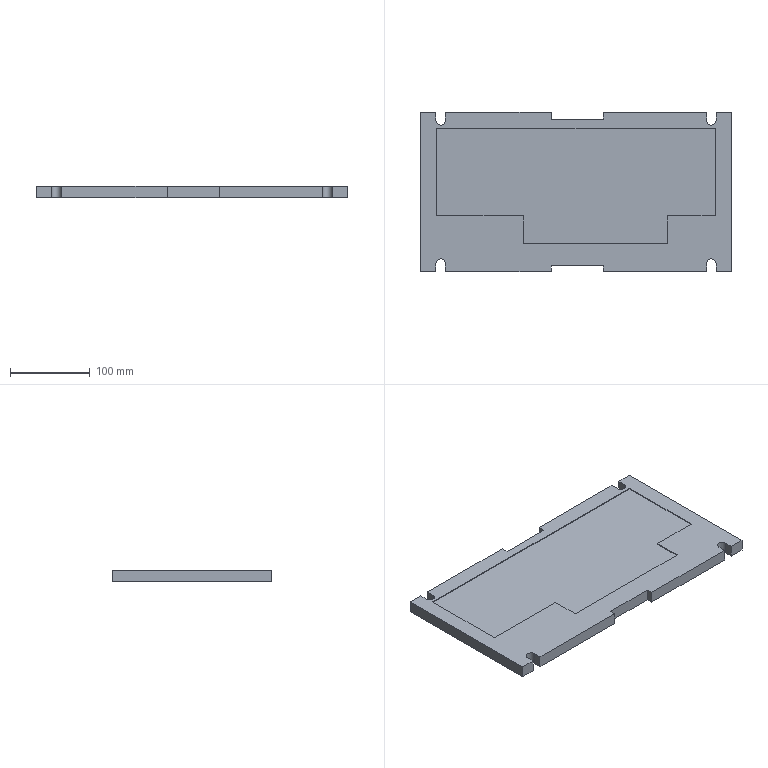Part | STEP file | MYT-A01-P07 | 1 solid | 39 faces | box 390 x 200 x 15 mm | volume 1098768 mm3 | plane 35 | cylinder 4 | commonest cylinder face diameters 12 x4
STEP:
#1=CARTESIAN_POINT('',(-31.137,100.,0.));
#2=VERTEX_POINT('',#1);
#3=CARTESIAN_POINT('',(-164.,100.,0.));
#4=VERTEX_POINT('',#3);
#5=CARTESIAN_POINT('',(-195.,100.,0.));
#6=DIRECTION('',(-1.,0.,0.));
#7=VECTOR('',#6,1000.);
#8=LINE('',#5,#7);
#9=EDGE_CURVE('',#2,#4,#8,.T.);
#10=ORIENTED_EDGE('',*,*,#9,.T.);
#11=CARTESIAN_POINT('',(-164.,100.,15.));
#12=VERTEX_POINT('',#11);
#13=CARTESIAN_POINT('',(-164.,100.,15.));
#14=DIRECTION('',(0.,0.,1.));
#15=VECTOR('',#14,1000.);
#16=LINE('',#13,#15);
#17=EDGE_CURVE('',#4,#12,#16,.T.);
#18=ORIENTED_EDGE('',*,*,#17,.T.);
#19=CARTESIAN_POINT('',(-31.137,100.,15.));
#20=VERTEX_POINT('',#19);
#21=CARTESIAN_POINT('',(-195.,100.,15.));
#22=DIRECTION('',(-1.,0.,0.));
#23=VECTOR('',#22,1000.);
#24=LINE('',#21,#23);
#25=EDGE_CURVE('',#20,#12,#24,.T.);
#26=ORIENTED_EDGE('',*,*,#25,.F.);
#27=CARTESIAN_POINT('',(-31.137,100.,15.));
#28=DIRECTION('',(0.,0.,-1.));
#29=VECTOR('',#28,1000.);
#30=LINE('',#27,#29);
#31=EDGE_CURVE('',#20,#2,#30,.T.);
#32=ORIENTED_EDGE('',*,*,#31,.T.);
#33=EDGE_LOOP('',(#10,#18,#26,#32));
#34=FACE_OUTER_BOUND('',#33,.T.);
#35=CARTESIAN_POINT('',(-195.,100.,15.));
#36=DIRECTION('',(0.,-1.,0.));
#37=DIRECTION('',(0.,0.,-1.));
#38=AXIS2_PLACEMENT_3D('',#35,#36,#37);
#39=PLANE('',#38);
#40=ADVANCED_FACE('',(#34),#39,.F.);
#41=CARTESIAN_POINT('',(-195.,-100.,0.));
#42=VERTEX_POINT('',#41);
#43=CARTESIAN_POINT('',(-176.,-100.,0.));
#44=VERTEX_POINT('',#43);
#45=CARTESIAN_POINT('',(-195.,-100.,0.));
#46=DIRECTION('',(1.,0.,0.));
#47=VECTOR('',#46,1000.);
#48=LINE('',#45,#47);
#49=EDGE_CURVE('',#42,#44,#48,.T.);
#50=ORIENTED_EDGE('',*,*,#49,.T.);
#51=CARTESIAN_POINT('',(-176.,-100.,15.));
#52=VERTEX_POINT('',#51);
#53=CARTESIAN_POINT('',(-176.,-100.,15.));
#54=DIRECTION('',(0.,0.,1.));
#55=VECTOR('',#54,1000.);
#56=LINE('',#53,#55);
#57=EDGE_CURVE('',#44,#52,#56,.T.);
#58=ORIENTED_EDGE('',*,*,#57,.T.);
#59=CARTESIAN_POINT('',(-195.,-100.,15.));
#60=VERTEX_POINT('',#59);
#61=CARTESIAN_POINT('',(-195.,-100.,15.));
#62=DIRECTION('',(1.,0.,0.));
#63=VECTOR('',#62,1000.);
#64=LINE('',#61,#63);
#65=EDGE_CURVE('',#60,#52,#64,.T.);
#66=ORIENTED_EDGE('',*,*,#65,.F.);
#67=CARTESIAN_POINT('',(-195.,-100.,15.));
#68=DIRECTION('',(0.,0.,-1.));
#69=VECTOR('',#68,1000.);
#70=LINE('',#67,#69);
#71=EDGE_CURVE('',#60,#42,#70,.T.);
#72=ORIENTED_EDGE('',*,*,#71,.T.);
#73=EDGE_LOOP('',(#50,#58,#66,#72));
#74=FACE_OUTER_BOUND('',#73,.T.);
#75=CARTESIAN_POINT('',(-195.,-100.,15.));
#76=DIRECTION('',(0.,1.,0.));
#77=DIRECTION('',(0.,0.,1.));
#78=AXIS2_PLACEMENT_3D('',#75,#76,#77);
#79=PLANE('',#78);
#80=ADVANCED_FACE('',(#74),#79,.F.);
#81=CARTESIAN_POINT('',(195.,100.,0.));
#82=VERTEX_POINT('',#81);
#83=CARTESIAN_POINT('',(176.,100.,0.));
#84=VERTEX_POINT('',#83);
#85=CARTESIAN_POINT('',(-195.,100.,0.));
#86=DIRECTION('',(-1.,0.,0.));
#87=VECTOR('',#86,1000.);
#88=LINE('',#85,#87);
#89=EDGE_CURVE('',#82,#84,#88,.T.);
#90=ORIENTED_EDGE('',*,*,#89,.T.);
#91=CARTESIAN_POINT('',(176.,100.,15.));
#92=VERTEX_POINT('',#91);
#93=CARTESIAN_POINT('',(176.,100.,15.));
#94=DIRECTION('',(0.,0.,1.));
#95=VECTOR('',#94,1000.);
#96=LINE('',#93,#95);
#97=EDGE_CURVE('',#84,#92,#96,.T.);
#98=ORIENTED_EDGE('',*,*,#97,.T.);
#99=CARTESIAN_POINT('',(195.,100.,15.));
#100=VERTEX_POINT('',#99);
#101=CARTESIAN_POINT('',(-195.,100.,15.));
#102=DIRECTION('',(-1.,0.,0.));
#103=VECTOR('',#102,1000.);
#104=LINE('',#101,#103);
#105=EDGE_CURVE('',#100,#92,#104,.T.);
#106=ORIENTED_EDGE('',*,*,#105,.F.);
#107=CARTESIAN_POINT('',(195.,100.,15.));
#108=DIRECTION('',(0.,0.,-1.));
#109=VECTOR('',#108,1000.);
#110=LINE('',#107,#109);
#111=EDGE_CURVE('',#100,#82,#110,.T.);
#112=ORIENTED_EDGE('',*,*,#111,.T.);
#113=EDGE_LOOP('',(#90,#98,#106,#112));
#114=FACE_OUTER_BOUND('',#113,.T.);
#115=CARTESIAN_POINT('',(-195.,100.,15.));
#116=DIRECTION('',(0.,-1.,0.));
#117=DIRECTION('',(0.,0.,-1.));
#118=AXIS2_PLACEMENT_3D('',#115,#116,#117);
#119=PLANE('',#118);
#120=ADVANCED_FACE('',(#114),#119,.F.);
#121=CARTESIAN_POINT('',(34.454,-100.,0.));
#122=VERTEX_POINT('',#121);
#123=CARTESIAN_POINT('',(164.,-100.,0.));
#124=VERTEX_POINT('',#123);
#125=CARTESIAN_POINT('',(-195.,-100.,0.));
#126=DIRECTION('',(1.,0.,0.));
#127=VECTOR('',#126,1000.);
#128=LINE('',#125,#127);
#129=EDGE_CURVE('',#122,#124,#128,.T.);
#130=ORIENTED_EDGE('',*,*,#129,.T.);
#131=CARTESIAN_POINT('',(164.,-100.,15.));
#132=VERTEX_POINT('',#131);
#133=CARTESIAN_POINT('',(164.,-100.,15.));
#134=DIRECTION('',(0.,0.,1.));
#135=VECTOR('',#134,1000.);
#136=LINE('',#133,#135);
#137=EDGE_CURVE('',#124,#132,#136,.T.);
#138=ORIENTED_EDGE('',*,*,#137,.T.);
#139=CARTESIAN_POINT('',(34.454,-100.,15.));
#140=VERTEX_POINT('',#139);
#141=CARTESIAN_POINT('',(-195.,-100.,15.));
#142=DIRECTION('',(1.,0.,0.));
#143=VECTOR('',#142,1000.);
#144=LINE('',#141,#143);
#145=EDGE_CURVE('',#140,#132,#144,.T.);
#146=ORIENTED_EDGE('',*,*,#145,.F.);
#147=CARTESIAN_POINT('',(34.454,-100.,15.));
#148=DIRECTION('',(0.,0.,-1.));
#149=VECTOR('',#148,1000.);
#150=LINE('',#147,#149);
#151=EDGE_CURVE('',#140,#122,#150,.T.);
#152=ORIENTED_EDGE('',*,*,#151,.T.);
#153=EDGE_LOOP('',(#130,#138,#146,#152));
#154=FACE_OUTER_BOUND('',#153,.T.);
#155=CARTESIAN_POINT('',(-195.,-100.,15.));
#156=DIRECTION('',(0.,1.,0.));
#157=DIRECTION('',(0.,0.,1.));
#158=AXIS2_PLACEMENT_3D('',#155,#156,#157);
#159=PLANE('',#158);
#160=ADVANCED_FACE('',(#154),#159,.F.);
#161=CARTESIAN_POINT('',(-176.,100.,15.));
#162=VERTEX_POINT('',#161);
#163=CARTESIAN_POINT('',(-195.,100.,15.));
#164=VERTEX_POINT('',#163);
#165=CARTESIAN_POINT('',(-195.,100.,15.));
#166=DIRECTION('',(-1.,0.,0.));
#167=VECTOR('',#166,1000.);
#168=LINE('',#165,#167);
#169=EDGE_CURVE('',#162,#164,#168,.T.);
#170=ORIENTED_EDGE('',*,*,#169,.F.);
#171=CARTESIAN_POINT('',(-176.,100.,0.));
#172=VERTEX_POINT('',#171);
#173=CARTESIAN_POINT('',(-176.,100.,15.));
#174=DIRECTION('',(0.,0.,-1.));
#175=VECTOR('',#174,1000.);
#176=LINE('',#173,#175);
#177=EDGE_CURVE('',#162,#172,#176,.T.);
#178=ORIENTED_EDGE('',*,*,#177,.T.);
#179=CARTESIAN_POINT('',(-195.,100.,0.));
#180=VERTEX_POINT('',#179);
#181=CARTESIAN_POINT('',(-195.,100.,0.));
#182=DIRECTION('',(-1.,0.,0.));
#183=VECTOR('',#182,1000.);
#184=LINE('',#181,#183);
#185=EDGE_CURVE('',#172,#180,#184,.T.);
#186=ORIENTED_EDGE('',*,*,#185,.T.);
#187=CARTESIAN_POINT('',(-195.,100.,15.));
#188=DIRECTION('',(0.,0.,-1.));
#189=VECTOR('',#188,1000.);
#190=LINE('',#187,#189);
#191=EDGE_CURVE('',#164,#180,#190,.T.);
#192=ORIENTED_EDGE('',*,*,#191,.F.);
#193=EDGE_LOOP('',(#170,#178,#186,#192));
#194=FACE_OUTER_BOUND('',#193,.T.);
#195=CARTESIAN_POINT('',(-195.,100.,15.));
#196=DIRECTION('',(0.,-1.,0.));
#197=DIRECTION('',(0.,0.,-1.));
#198=AXIS2_PLACEMENT_3D('',#195,#196,#197);
#199=PLANE('',#198);
#200=ADVANCED_FACE('',(#194),#199,.F.);
#201=CARTESIAN_POINT('',(-164.,-100.,15.));
#202=VERTEX_POINT('',#201);
#203=CARTESIAN_POINT('',(-31.137,-100.,15.));
#204=VERTEX_POINT('',#203);
#205=CARTESIAN_POINT('',(-195.,-100.,15.));
#206=DIRECTION('',(1.,0.,0.));
#207=VECTOR('',#206,1000.);
#208=LINE('',#205,#207);
#209=EDGE_CURVE('',#202,#204,#208,.T.);
#210=ORIENTED_EDGE('',*,*,#209,.F.);
#211=CARTESIAN_POINT('',(-164.,-100.,0.));
#212=VERTEX_POINT('',#211);
#213=CARTESIAN_POINT('',(-164.,-100.,15.));
#214=DIRECTION('',(0.,0.,-1.));
#215=VECTOR('',#214,1000.);
#216=LINE('',#213,#215);
#217=EDGE_CURVE('',#202,#212,#216,.T.);
#218=ORIENTED_EDGE('',*,*,#217,.T.);
#219=CARTESIAN_POINT('',(-31.137,-100.,0.));
#220=VERTEX_POINT('',#219);
#221=CARTESIAN_POINT('',(-195.,-100.,0.));
#222=DIRECTION('',(1.,0.,0.));
#223=VECTOR('',#222,1000.);
#224=LINE('',#221,#223);
#225=EDGE_CURVE('',#212,#220,#224,.T.);
#226=ORIENTED_EDGE('',*,*,#225,.T.);
#227=CARTESIAN_POINT('',(-31.137,-100.,15.));
#228=DIRECTION('',(0.,0.,1.));
#229=VECTOR('',#228,1000.);
#230=LINE('',#227,#229);
#231=EDGE_CURVE('',#220,#204,#230,.T.);
#232=ORIENTED_EDGE('',*,*,#231,.T.);
#233=EDGE_LOOP('',(#210,#218,#226,#232));
#234=FACE_OUTER_BOUND('',#233,.T.);
#235=CARTESIAN_POINT('',(-195.,-100.,15.));
#236=DIRECTION('',(0.,1.,0.));
#237=DIRECTION('',(0.,0.,1.));
#238=AXIS2_PLACEMENT_3D('',#235,#236,#237);
#239=PLANE('',#238);
#240=ADVANCED_FACE('',(#234),#239,.F.);
#241=CARTESIAN_POINT('',(195.,-100.,0.));
#242=VERTEX_POINT('',#241);
#243=CARTESIAN_POINT('',(195.,100.,0.));
#244=DIRECTION('',(0.,1.,0.));
#245=VECTOR('',#244,1000.);
#246=LINE('',#243,#245);
#247=EDGE_CURVE('',#242,#82,#246,.T.);
#248=ORIENTED_EDGE('',*,*,#247,.T.);
#249=ORIENTED_EDGE('',*,*,#111,.F.);
#250=CARTESIAN_POINT('',(195.,-100.,15.));
#251=VERTEX_POINT('',#250);
#252=CARTESIAN_POINT('',(195.,100.,15.));
#253=DIRECTION('',(0.,1.,0.));
#254=VECTOR('',#253,1000.);
#255=LINE('',#252,#254);
#256=EDGE_CURVE('',#251,#100,#255,.T.);
#257=ORIENTED_EDGE('',*,*,#256,.F.);
#258=CARTESIAN_POINT('',(195.,-100.,15.));
#259=DIRECTION('',(0.,0.,-1.));
#260=VECTOR('',#259,1000.);
#261=LINE('',#258,#260);
#262=EDGE_CURVE('',#251,#242,#261,.T.);
#263=ORIENTED_EDGE('',*,*,#262,.T.);
#264=EDGE_LOOP('',(#248,#249,#257,#263));
#265=FACE_OUTER_BOUND('',#264,.T.);
#266=CARTESIAN_POINT('',(195.,100.,15.));
#267=DIRECTION('',(-1.,0.,0.));
#268=DIRECTION('',(0.,0.,1.));
#269=AXIS2_PLACEMENT_3D('',#266,#267,#268);
#270=PLANE('',#269);
#271=ADVANCED_FACE('',(#265),#270,.F.);
#272=CARTESIAN_POINT('',(164.,100.,15.));
#273=VERTEX_POINT('',#272);
#274=CARTESIAN_POINT('',(34.454,100.,15.));
#275=VERTEX_POINT('',#274);
#276=CARTESIAN_POINT('',(-195.,100.,15.));
#277=DIRECTION('',(-1.,0.,0.));
#278=VECTOR('',#277,1000.);
#279=LINE('',#276,#278);
#280=EDGE_CURVE('',#273,#275,#279,.T.);
#281=ORIENTED_EDGE('',*,*,#280,.F.);
#282=CARTESIAN_POINT('',(164.,100.,0.));
#283=VERTEX_POINT('',#282);
#284=CARTESIAN_POINT('',(164.,100.,15.));
#285=DIRECTION('',(0.,0.,-1.));
#286=VECTOR('',#285,1000.);
#287=LINE('',#284,#286);
#288=EDGE_CURVE('',#273,#283,#287,.T.);
#289=ORIENTED_EDGE('',*,*,#288,.T.);
#290=CARTESIAN_POINT('',(34.454,100.,0.));
#291=VERTEX_POINT('',#290);
#292=CARTESIAN_POINT('',(-195.,100.,0.));
#293=DIRECTION('',(-1.,0.,0.));
#294=VECTOR('',#293,1000.);
#295=LINE('',#292,#294);
#296=EDGE_CURVE('',#283,#291,#295,.T.);
#297=ORIENTED_EDGE('',*,*,#296,.T.);
#298=CARTESIAN_POINT('',(34.454,100.,15.));
#299=DIRECTION('',(0.,0.,1.));
#300=VECTOR('',#299,1000.);
#301=LINE('',#298,#300);
#302=EDGE_CURVE('',#291,#275,#301,.T.);
#303=ORIENTED_EDGE('',*,*,#302,.T.);
#304=EDGE_LOOP('',(#281,#289,#297,#303));
#305=FACE_OUTER_BOUND('',#304,.T.);
#306=CARTESIAN_POINT('',(-195.,100.,15.));
#307=DIRECTION('',(0.,-1.,0.));
#308=DIRECTION('',(0.,0.,-1.));
#309=AXIS2_PLACEMENT_3D('',#306,#307,#308);
#310=PLANE('',#309);
#311=ADVANCED_FACE('',(#305),#310,.F.);
#312=CARTESIAN_POINT('',(-195.,100.,0.));
#313=DIRECTION('',(0.,-1.,0.));
#314=VECTOR('',#313,1000.);
#315=LINE('',#312,#314);
#316=EDGE_CURVE('',#180,#42,#315,.T.);
#317=ORIENTED_EDGE('',*,*,#316,.T.);
#318=ORIENTED_EDGE('',*,*,#71,.F.);
#319=CARTESIAN_POINT('',(-195.,100.,15.));
#320=DIRECTION('',(0.,-1.,0.));
#321=VECTOR('',#320,1000.);
#322=LINE('',#319,#321);
#323=EDGE_CURVE('',#164,#60,#322,.T.);
#324=ORIENTED_EDGE('',*,*,#323,.F.);
#325=ORIENTED_EDGE('',*,*,#191,.T.);
#326=EDGE_LOOP('',(#317,#318,#324,#325));
#327=FACE_OUTER_BOUND('',#326,.T.);
#328=CARTESIAN_POINT('',(-195.,100.,15.));
#329=DIRECTION('',(1.,0.,0.));
#330=DIRECTION('',(0.,1.,0.));
#331=AXIS2_PLACEMENT_3D('',#328,#329,#330);
#332=PLANE('',#331);
#333=ADVANCED_FACE('',(#327),#332,.F.);
#334=CARTESIAN_POINT('',(176.,-100.,15.));
#335=VERTEX_POINT('',#334);
#336=CARTESIAN_POINT('',(-195.,-100.,15.));
#337=DIRECTION('',(1.,0.,0.));
#338=VECTOR('',#337,1000.);
#339=LINE('',#336,#338);
#340=EDGE_CURVE('',#335,#251,#339,.T.);
#341=ORIENTED_EDGE('',*,*,#340,.F.);
#342=CARTESIAN_POINT('',(176.,-100.,0.));
#343=VERTEX_POINT('',#342);
#344=CARTESIAN_POINT('',(176.,-100.,15.));
#345=DIRECTION('',(0.,0.,-1.));
#346=VECTOR('',#345,1000.);
#347=LINE('',#344,#346);
#348=EDGE_CURVE('',#335,#343,#347,.T.);
#349=ORIENTED_EDGE('',*,*,#348,.T.);
#350=CARTESIAN_POINT('',(-195.,-100.,0.));
#351=DIRECTION('',(1.,0.,0.));
#352=VECTOR('',#351,1000.);
#353=LINE('',#350,#352);
#354=EDGE_CURVE('',#343,#242,#353,.T.);
#355=ORIENTED_EDGE('',*,*,#354,.T.);
#356=ORIENTED_EDGE('',*,*,#262,.F.);
#357=EDGE_LOOP('',(#341,#349,#355,#356));
#358=FACE_OUTER_BOUND('',#357,.T.);
#359=CARTESIAN_POINT('',(-195.,-100.,15.));
#360=DIRECTION('',(0.,1.,0.));
#361=DIRECTION('',(0.,0.,1.));
#362=AXIS2_PLACEMENT_3D('',#359,#360,#361);
#363=PLANE('',#362);
#364=ADVANCED_FACE('',(#358),#363,.F.);
#365=CARTESIAN_POINT('',(-176.,-90.,15.));
#366=VERTEX_POINT('',#365);
#367=CARTESIAN_POINT('',(-176.,-110.,15.));
#368=DIRECTION('',(0.,-1.,0.));
#369=VECTOR('',#368,1000.);
#370=LINE('',#367,#369);
#371=EDGE_CURVE('',#366,#52,#370,.T.);
#372=ORIENTED_EDGE('',*,*,#371,.F.);
#373=CARTESIAN_POINT('',(-164.,-90.,15.));
#374=VERTEX_POINT('',#373);
#375=CARTESIAN_POINT('',(-170.,-90.,15.));
#376=DIRECTION('',(0.,0.,1.));
#377=DIRECTION('',(-1.,0.,0.));
#378=AXIS2_PLACEMENT_3D('',#375,#376,#377);
#379=CIRCLE('',#378,6.);
#380=EDGE_CURVE('',#374,#366,#379,.T.);
#381=ORIENTED_EDGE('',*,*,#380,.F.);
#382=CARTESIAN_POINT('',(-164.,-110.,15.));
#383=DIRECTION('',(0.,1.,0.));
#384=VECTOR('',#383,1000.);
#385=LINE('',#382,#384);
#386=EDGE_CURVE('',#202,#374,#385,.T.);
#387=ORIENTED_EDGE('',*,*,#386,.F.);
#388=ORIENTED_EDGE('',*,*,#209,.T.);
#389=CARTESIAN_POINT('',(-31.137,-92.567,15.));
#390=VERTEX_POINT('',#389);
#391=CARTESIAN_POINT('',(-31.137,-118.233,15.));
#392=DIRECTION('',(0.,-1.,0.));
#393=VECTOR('',#392,1000.);
#394=LINE('',#391,#393);
#395=EDGE_CURVE('',#390,#204,#394,.T.);
#396=ORIENTED_EDGE('',*,*,#395,.F.);
#397=CARTESIAN_POINT('',(34.454,-92.567,15.));
#398=VERTEX_POINT('',#397);
#399=CARTESIAN_POINT('',(-31.137,-92.567,15.));
#400=DIRECTION('',(-1.,0.,0.));
#401=VECTOR('',#400,1000.);
#402=LINE('',#399,#401);
#403=EDGE_CURVE('',#398,#390,#402,.T.);
#404=ORIENTED_EDGE('',*,*,#403,.F.);
#405=CARTESIAN_POINT('',(34.454,-118.233,15.));
#406=DIRECTION('',(0.,1.,0.));
#407=VECTOR('',#406,1000.);
#408=LINE('',#405,#407);
#409=EDGE_CURVE('',#140,#398,#408,.T.);
#410=ORIENTED_EDGE('',*,*,#409,.F.);
#411=ORIENTED_EDGE('',*,*,#145,.T.);
#412=CARTESIAN_POINT('',(164.,-90.,15.));
#413=VERTEX_POINT('',#412);
#414=CARTESIAN_POINT('',(164.,-110.,15.));
#415=DIRECTION('',(0.,-1.,0.));
#416=VECTOR('',#415,1000.);
#417=LINE('',#414,#416);
#418=EDGE_CURVE('',#413,#132,#417,.T.);
#419=ORIENTED_EDGE('',*,*,#418,.F.);
#420=CARTESIAN_POINT('',(176.,-90.,15.));
#421=VERTEX_POINT('',#420);
#422=CARTESIAN_POINT('',(170.,-90.,15.));
#423=DIRECTION('',(0.,0.,1.));
#424=DIRECTION('',(-1.,0.,0.));
#425=AXIS2_PLACEMENT_3D('',#422,#423,#424);
#426=CIRCLE('',#425,6.);
#427=EDGE_CURVE('',#421,#413,#426,.T.);
#428=ORIENTED_EDGE('',*,*,#427,.F.);
#429=CARTESIAN_POINT('',(176.,-110.,15.));
#430=DIRECTION('',(0.,1.,0.));
#431=VECTOR('',#430,1000.);
#432=LINE('',#429,#431);
#433=EDGE_CURVE('',#335,#421,#432,.T.);
#434=ORIENTED_EDGE('',*,*,#433,.F.);
#435=ORIENTED_EDGE('',*,*,#340,.T.);
#436=ORIENTED_EDGE('',*,*,#256,.T.);
#437=ORIENTED_EDGE('',*,*,#105,.T.);
#438=CARTESIAN_POINT('',(176.,90.,15.));
#439=VERTEX_POINT('',#438);
#440=CARTESIAN_POINT('',(176.,110.,15.));
#441=DIRECTION('',(0.,1.,0.));
#442=VECTOR('',#441,1000.);
#443=LINE('',#440,#442);
#444=EDGE_CURVE('',#439,#92,#443,.T.);
#445=ORIENTED_EDGE('',*,*,#444,.F.);
#446=CARTESIAN_POINT('',(164.,90.,15.));
#447=VERTEX_POINT('',#446);
#448=CARTESIAN_POINT('',(170.,90.,15.));
#449=DIRECTION('',(0.,0.,1.));
#450=DIRECTION('',(1.,0.,0.));
#451=AXIS2_PLACEMENT_3D('',#448,#449,#450);
#452=CIRCLE('',#451,6.);
#453=EDGE_CURVE('',#447,#439,#452,.T.);
#454=ORIENTED_EDGE('',*,*,#453,.F.);
#455=CARTESIAN_POINT('',(164.,110.,15.));
#456=DIRECTION('',(0.,-1.,0.));
#457=VECTOR('',#456,1000.);
#458=LINE('',#455,#457);
#459=EDGE_CURVE('',#273,#447,#458,.T.);
#460=ORIENTED_EDGE('',*,*,#459,.F.);
#461=ORIENTED_EDGE('',*,*,#280,.T.);
#462=CARTESIAN_POINT('',(34.454,91.372,15.));
#463=VERTEX_POINT('',#462);
#464=CARTESIAN_POINT('',(34.454,110.859,15.));
#465=DIRECTION('',(0.,1.,0.));
#466=VECTOR('',#465,1000.);
#467=LINE('',#464,#466);
#468=EDGE_CURVE('',#463,#275,#467,.T.);
#469=ORIENTED_EDGE('',*,*,#468,.F.);
#470=CARTESIAN_POINT('',(-31.137,91.372,15.));
#471=VERTEX_POINT('',#470);
#472=CARTESIAN_POINT('',(-31.137,91.372,15.));
#473=DIRECTION('',(1.,0.,0.));
#474=VECTOR('',#473,1000.);
#475=LINE('',#472,#474);
#476=EDGE_CURVE('',#471,#463,#475,.T.);
#477=ORIENTED_EDGE('',*,*,#476,.F.);
#478=CARTESIAN_POINT('',(-31.137,110.859,15.));
#479=DIRECTION('',(0.,-1.,0.));
#480=VECTOR('',#479,1000.);
#481=LINE('',#478,#480);
#482=EDGE_CURVE('',#20,#471,#481,.T.);
#483=ORIENTED_EDGE('',*,*,#482,.F.);
#484=ORIENTED_EDGE('',*,*,#25,.T.);
#485=CARTESIAN_POINT('',(-164.,90.,15.));
#486=VERTEX_POINT('',#485);
#487=CARTESIAN_POINT('',(-164.,110.,15.));
#488=DIRECTION('',(0.,1.,0.));
#489=VECTOR('',#488,1000.);
#490=LINE('',#487,#489);
#491=EDGE_CURVE('',#486,#12,#490,.T.);
#492=ORIENTED_EDGE('',*,*,#491,.F.);
#493=CARTESIAN_POINT('',(-176.,90.,15.));
#494=VERTEX_POINT('',#493);
#495=CARTESIAN_POINT('',(-170.,90.,15.));
#496=DIRECTION('',(0.,0.,1.));
#497=DIRECTION('',(1.,0.,0.));
#498=AXIS2_PLACEMENT_3D('',#495,#496,#497);
#499=CIRCLE('',#498,6.);
#500=EDGE_CURVE('',#494,#486,#499,.T.);
#501=ORIENTED_EDGE('',*,*,#500,.F.);
#502=CARTESIAN_POINT('',(-176.,110.,15.));
#503=DIRECTION('',(0.,-1.,0.));
#504=VECTOR('',#503,1000.);
#505=LINE('',#502,#504);
#506=EDGE_CURVE('',#162,#494,#505,.T.);
#507=ORIENTED_EDGE('',*,*,#506,.F.);
#508=ORIENTED_EDGE('',*,*,#169,.T.);
#509=ORIENTED_EDGE('',*,*,#323,.T.);
#510=ORIENTED_EDGE('',*,*,#65,.T.);
#511=EDGE_LOOP('',(#372,#381,#387,#388,#396,#404,#410,#411,#419,#428,#434,#435,#436,#437,#445,#454,#460,#461,#469,#477,#483,#484,#492,#501,#507,#508,#509,#510));
#512=FACE_OUTER_BOUND('',#511,.T.);
#513=CARTESIAN_POINT('',(-175.,80.,15.));
#514=VERTEX_POINT('',#513);
#515=CARTESIAN_POINT('',(-175.,-30.,15.));
#516=VERTEX_POINT('',#515);
#517=CARTESIAN_POINT('',(-175.,80.,15.));
#518=DIRECTION('',(0.,-1.,0.));
#519=VECTOR('',#518,1000.);
#520=LINE('',#517,#519);
#521=EDGE_CURVE('',#514,#516,#520,.T.);
#522=ORIENTED_EDGE('',*,*,#521,.F.);
#523=CARTESIAN_POINT('',(175.,80.,15.));
#524=VERTEX_POINT('',#523);
#525=CARTESIAN_POINT('',(-175.,80.,15.));
#526=DIRECTION('',(-1.,0.,0.));
#527=VECTOR('',#526,1000.);
#528=LINE('',#525,#527);
#529=EDGE_CURVE('',#524,#514,#528,.T.);
#530=ORIENTED_EDGE('',*,*,#529,.F.);
#531=CARTESIAN_POINT('',(175.,-30.,15.));
#532=VERTEX_POINT('',#531);
#533=CARTESIAN_POINT('',(175.,80.,15.));
#534=DIRECTION('',(0.,1.,0.));
#535=VECTOR('',#534,1000.);
#536=LINE('',#533,#535);
#537=EDGE_CURVE('',#532,#524,#536,.T.);
#538=ORIENTED_EDGE('',*,*,#537,.F.);
#539=CARTESIAN_POINT('',(114.758,-30.,15.));
#540=VERTEX_POINT('',#539);
#541=CARTESIAN_POINT('',(114.758,-30.,15.));
#542=DIRECTION('',(1.,0.,0.));
#543=VECTOR('',#542,1000.);
#544=LINE('',#541,#543);
#545=EDGE_CURVE('',#540,#532,#544,.T.);
#546=ORIENTED_EDGE('',*,*,#545,.F.);
#547=CARTESIAN_POINT('',(114.758,-65.,15.));
#548=VERTEX_POINT('',#547);
#549=CARTESIAN_POINT('',(114.758,-30.,15.));
#550=DIRECTION('',(0.,1.,0.));
#551=VECTOR('',#550,1000.);
#552=LINE('',#549,#551);
#553=EDGE_CURVE('',#548,#540,#552,.T.);
#554=ORIENTED_EDGE('',*,*,#553,.F.);
#555=CARTESIAN_POINT('',(-66.313,-65.,15.));
#556=VERTEX_POINT('',#555);
#557=CARTESIAN_POINT('',(-66.313,-65.,15.));
#558=DIRECTION('',(1.,0.,0.));
#559=VECTOR('',#558,1000.);
#560=LINE('',#557,#559);
#561=EDGE_CURVE('',#556,#548,#560,.T.);
#562=ORIENTED_EDGE('',*,*,#561,.F.);
#563=CARTESIAN_POINT('',(-66.313,-30.,15.));
#564=VERTEX_POINT('',#563);
#565=CARTESIAN_POINT('',(-66.313,-30.,15.));
#566=DIRECTION('',(0.,-1.,0.));
#567=VECTOR('',#566,1000.);
#568=LINE('',#565,#567);
#569=EDGE_CURVE('',#564,#556,#568,.T.);
#570=ORIENTED_EDGE('',*,*,#569,.F.);
#571=CARTESIAN_POINT('',(-175.,-30.,15.));
#572=DIRECTION('',(1.,0.,0.));
#573=VECTOR('',#572,1000.);
#574=LINE('',#571,#573);
#575=EDGE_CURVE('',#516,#564,#574,.T.);
#576=ORIENTED_EDGE('',*,*,#575,.F.);
#577=EDGE_LOOP('',(#522,#530,#538,#546,#554,#562,#570,#576));
#578=FACE_BOUND('',#577,.T.);
#579=CARTESIAN_POINT('',(0.,0.,15.));
#580=DIRECTION('',(0.,0.,1.));
#581=DIRECTION('',(1.,0.,0.));
#582=AXIS2_PLACEMENT_3D('',#579,#580,#581);
#583=PLANE('',#582);
#584=ADVANCED_FACE('',(#512,#578),#583,.T.);
#585=CARTESIAN_POINT('',(-164.,-90.,0.));
#586=VERTEX_POINT('',#585);
#587=CARTESIAN_POINT('',(-176.,-90.,0.));
#588=VERTEX_POINT('',#587);
#589=CARTESIAN_POINT('',(-170.,-90.,0.));
#590=DIRECTION('',(0.,0.,1.));
#591=DIRECTION('',(-1.,0.,0.));
#592=AXIS2_PLACEMENT_3D('',#589,#590,#591);
#593=CIRCLE('',#592,6.);
#594=EDGE_CURVE('',#586,#588,#593,.T.);
#595=ORIENTED_EDGE('',*,*,#594,.T.);
#596=CARTESIAN_POINT('',(-176.,-110.,0.));
#597=DIRECTION('',(0.,-1.,0.));
#598=VECTOR('',#597,1000.);
#599=LINE('',#596,#598);
#600=EDGE_CURVE('',#588,#44,#599,.T.);
#601=ORIENTED_EDGE('',*,*,#600,.T.);
#602=ORIENTED_EDGE('',*,*,#49,.F.);
#603=ORIENTED_EDGE('',*,*,#316,.F.);
#604=ORIENTED_EDGE('',*,*,#185,.F.);
#605=CARTESIAN_POINT('',(-176.,90.,0.));
#606=VERTEX_POINT('',#605);
#607=CARTESIAN_POINT('',(-176.,0.,0.));
#608=DIRECTION('',(0.,-1.,0.));
#609=VECTOR('',#608,1000.);
#610=LINE('',#607,#609);
#611=EDGE_CURVE('',#172,#606,#610,.T.);
#612=ORIENTED_EDGE('',*,*,#611,.T.);
#613=CARTESIAN_POINT('',(-164.,90.,0.));
#614=VERTEX_POINT('',#613);
#615=CARTESIAN_POINT('',(-170.,90.,0.));
#616=DIRECTION('',(0.,0.,1.));
#617=DIRECTION('',(1.,0.,0.));
#618=AXIS2_PLACEMENT_3D('',#615,#616,#617);
#619=CIRCLE('',#618,6.);
#620=EDGE_CURVE('',#606,#614,#619,.T.);
#621=ORIENTED_EDGE('',*,*,#620,.T.);
#622=CARTESIAN_POINT('',(-164.,110.,0.));
#623=DIRECTION('',(0.,1.,0.));
#624=VECTOR('',#623,1000.);
#625=LINE('',#622,#624);
#626=EDGE_CURVE('',#614,#4,#625,.T.);
#627=ORIENTED_EDGE('',*,*,#626,.T.);
#628=ORIENTED_EDGE('',*,*,#9,.F.);
#629=CARTESIAN_POINT('',(-31.137,91.372,0.));
#630=VERTEX_POINT('',#629);
#631=CARTESIAN_POINT('',(-31.137,0.,0.));
#632=DIRECTION('',(0.,-1.,0.));
#633=VECTOR('',#632,1000.);
#634=LINE('',#631,#633);
#635=EDGE_CURVE('',#2,#630,#634,.T.);
#636=ORIENTED_EDGE('',*,*,#635,.T.);
#637=CARTESIAN_POINT('',(34.454,91.372,0.));
#638=VERTEX_POINT('',#637);
#639=CARTESIAN_POINT('',(0.,91.372,0.));
#640=DIRECTION('',(1.,0.,0.));
#641=VECTOR('',#640,1000.);
#642=LINE('',#639,#641);
#643=EDGE_CURVE('',#630,#638,#642,.T.);
#644=ORIENTED_EDGE('',*,*,#643,.T.);
#645=CARTESIAN_POINT('',(34.454,0.,0.));
#646=DIRECTION('',(0.,1.,0.));
#647=VECTOR('',#646,1000.);
#648=LINE('',#645,#647);
#649=EDGE_CURVE('',#638,#291,#648,.T.);
#650=ORIENTED_EDGE('',*,*,#649,.T.);
#651=ORIENTED_EDGE('',*,*,#296,.F.);
#652=CARTESIAN_POINT('',(164.,90.,0.));
#653=VERTEX_POINT('',#652);
#654=CARTESIAN_POINT('',(164.,0.,0.));
#655=DIRECTION('',(0.,-1.,0.));
#656=VECTOR('',#655,1000.);
#657=LINE('',#654,#656);
#658=EDGE_CURVE('',#283,#653,#657,.T.);
#659=ORIENTED_EDGE('',*,*,#658,.T.);
#660=CARTESIAN_POINT('',(176.,90.,0.));
#661=VERTEX_POINT('',#660);
#662=CARTESIAN_POINT('',(170.,90.,0.));
#663=DIRECTION('',(0.,0.,1.));
#664=DIRECTION('',(1.,0.,0.));
#665=AXIS2_PLACEMENT_3D('',#662,#663,#664);
#666=CIRCLE('',#665,6.);
#667=EDGE_CURVE('',#653,#661,#666,.T.);
#668=ORIENTED_EDGE('',*,*,#667,.T.);
#669=CARTESIAN_POINT('',(176.,110.,0.));
#670=DIRECTION('',(0.,1.,0.));
#671=VECTOR('',#670,1000.);
#672=LINE('',#669,#671);
#673=EDGE_CURVE('',#661,#84,#672,.T.);
#674=ORIENTED_EDGE('',*,*,#673,.T.);
#675=ORIENTED_EDGE('',*,*,#89,.F.);
#676=ORIENTED_EDGE('',*,*,#247,.F.);
#677=ORIENTED_EDGE('',*,*,#354,.F.);
#678=CARTESIAN_POINT('',(176.,-90.,0.));
#679=VERTEX_POINT('',#678);
#680=CARTESIAN_POINT('',(176.,0.,0.));
#681=DIRECTION('',(0.,1.,0.));
#682=VECTOR('',#681,1000.);
#683=LINE('',#680,#682);
#684=EDGE_CURVE('',#343,#679,#683,.T.);
#685=ORIENTED_EDGE('',*,*,#684,.T.);
#686=CARTESIAN_POINT('',(164.,-90.,0.));
#687=VERTEX_POINT('',#686);
#688=CARTESIAN_POINT('',(170.,-90.,0.));
#689=DIRECTION('',(0.,0.,1.));
#690=DIRECTION('',(-1.,0.,0.));
#691=AXIS2_PLACEMENT_3D('',#688,#689,#690);
#692=CIRCLE('',#691,6.);
#693=EDGE_CURVE('',#679,#687,#692,.T.);
#694=ORIENTED_EDGE('',*,*,#693,.T.);
#695=CARTESIAN_POINT('',(164.,-110.,0.));
#696=DIRECTION('',(0.,-1.,0.));
#697=VECTOR('',#696,1000.);
#698=LINE('',#695,#697);
#699=EDGE_CURVE('',#687,#124,#698,.T.);
#700=ORIENTED_EDGE('',*,*,#699,.T.);
#701=ORIENTED_EDGE('',*,*,#129,.F.);
#702=CARTESIAN_POINT('',(34.454,-92.567,0.));
#703=VERTEX_POINT('',#702);
#704=CARTESIAN_POINT('',(34.454,0.,0.));
#705=DIRECTION('',(0.,1.,0.));
#706=VECTOR('',#705,1000.);
#707=LINE('',#704,#706);
#708=EDGE_CURVE('',#122,#703,#707,.T.);
#709=ORIENTED_EDGE('',*,*,#708,.T.);
#710=CARTESIAN_POINT('',(-31.137,-92.567,0.));
#711=VERTEX_POINT('',#710);
#712=CARTESIAN_POINT('',(0.,-92.567,0.));
#713=DIRECTION('',(-1.,0.,0.));
#714=VECTOR('',#713,1000.);
#715=LINE('',#712,#714);
#716=EDGE_CURVE('',#703,#711,#715,.T.);
#717=ORIENTED_EDGE('',*,*,#716,.T.);
#718=CARTESIAN_POINT('',(-31.137,0.,0.));
#719=DIRECTION('',(0.,-1.,0.));
#720=VECTOR('',#719,1000.);
#721=LINE('',#718,#720);
#722=EDGE_CURVE('',#711,#220,#721,.T.);
#723=ORIENTED_EDGE('',*,*,#722,.T.);
#724=ORIENTED_EDGE('',*,*,#225,.F.);
#725=CARTESIAN_POINT('',(-164.,0.,0.));
#726=DIRECTION('',(0.,1.,0.));
#727=VECTOR('',#726,1000.);
#728=LINE('',#725,#727);
#729=EDGE_CURVE('',#212,#586,#728,.T.);
#730=ORIENTED_EDGE('',*,*,#729,.T.);
#731=EDGE_LOOP('',(#595,#601,#602,#603,#604,#612,#621,#627,#628,#636,#644,#650,#651,#659,#668,#674,#675,#676,#677,#685,#694,#700,#701,#709,#717,#723,#724,#730));
#732=FACE_OUTER_BOUND('',#731,.T.);
#733=CARTESIAN_POINT('',(0.,0.,0.));
#734=DIRECTION('',(0.,0.,1.));
#735=DIRECTION('',(1.,0.,0.));
#736=AXIS2_PLACEMENT_3D('',#733,#734,#735);
#737=PLANE('',#736);
#738=ADVANCED_FACE('',(#732),#737,.F.);
#739=ORIENTED_EDGE('',*,*,#521,.T.);
#740=CARTESIAN_POINT('',(-175.,-30.,14.));
#741=VERTEX_POINT('',#740);
#742=CARTESIAN_POINT('',(-175.,-30.,14.));
#743=DIRECTION('',(0.,0.,1.));
#744=VECTOR('',#743,1000.);
#745=LINE('',#742,#744);
#746=EDGE_CURVE('',#741,#516,#745,.T.);
#747=ORIENTED_EDGE('',*,*,#746,.F.);
#748=CARTESIAN_POINT('',(-175.,80.,14.));
#749=VERTEX_POINT('',#748);
#750=CARTESIAN_POINT('',(-175.,80.,14.));
#751=DIRECTION('',(0.,-1.,0.));
#752=VECTOR('',#751,1000.);
#753=LINE('',#750,#752);
#754=EDGE_CURVE('',#749,#741,#753,.T.);
#755=ORIENTED_EDGE('',*,*,#754,.F.);
#756=CARTESIAN_POINT('',(-175.,80.,14.));
#757=DIRECTION('',(0.,0.,1.));
#758=VECTOR('',#757,1000.);
#759=LINE('',#756,#758);
#760=EDGE_CURVE('',#749,#514,#759,.T.);
#761=ORIENTED_EDGE('',*,*,#760,.T.);
#762=EDGE_LOOP('',(#739,#747,#755,#761));
#763=FACE_OUTER_BOUND('',#762,.T.);
#764=CARTESIAN_POINT('',(-175.,80.,14.));
#765=DIRECTION('',(-1.,0.,0.));
#766=DIRECTION('',(0.,0.,1.));
#767=AXIS2_PLACEMENT_3D('',#764,#765,#766);
#768=PLANE('',#767);
#769=ADVANCED_FACE('',(#763),#768,.F.);
#770=ORIENTED_EDGE('',*,*,#529,.T.);
#771=ORIENTED_EDGE('',*,*,#760,.F.);
#772=CARTESIAN_POINT('',(175.,80.,14.));
#773=VERTEX_POINT('',#772);
#774=CARTESIAN_POINT('',(-175.,80.,14.));
#775=DIRECTION('',(-1.,0.,0.));
#776=VECTOR('',#775,1000.);
#777=LINE('',#774,#776);
#778=EDGE_CURVE('',#773,#749,#777,.T.);
#779=ORIENTED_EDGE('',*,*,#778,.F.);
#780=CARTESIAN_POINT('',(175.,80.,14.));
#781=DIRECTION('',(0.,0.,1.));
#782=VECTOR('',#781,1000.);
#783=LINE('',#780,#782);
#784=EDGE_CURVE('',#773,#524,#783,.T.);
#785=ORIENTED_EDGE('',*,*,#784,.T.);
#786=EDGE_LOOP('',(#770,#771,#779,#785));
#787=FACE_OUTER_BOUND('',#786,.T.);
#788=CARTESIAN_POINT('',(-175.,80.,14.));
#789=DIRECTION('',(0.,1.,0.));
#790=DIRECTION('',(0.,0.,1.));
#791=AXIS2_PLACEMENT_3D('',#788,#789,#790);
#792=PLANE('',#791);
#793=ADVANCED_FACE('',(#787),#792,.F.);
#794=ORIENTED_EDGE('',*,*,#537,.T.);
#795=ORIENTED_EDGE('',*,*,#784,.F.);
#796=CARTESIAN_POINT('',(175.,-30.,14.));
#797=VERTEX_POINT('',#796);
#798=CARTESIAN_POINT('',(175.,80.,14.));
#799=DIRECTION('',(0.,1.,0.));
#800=VECTOR('',#799,1000.);
#801=LINE('',#798,#800);
#802=EDGE_CURVE('',#797,#773,#801,.T.);
#803=ORIENTED_EDGE('',*,*,#802,.F.);
#804=CARTESIAN_POINT('',(175.,-30.,14.));
#805=DIRECTION('',(0.,0.,1.));
#806=VECTOR('',#805,1000.);
#807=LINE('',#804,#806);
#808=EDGE_CURVE('',#797,#532,#807,.T.);
#809=ORIENTED_EDGE('',*,*,#808,.T.);
#810=EDGE_LOOP('',(#794,#795,#803,#809));
#811=FACE_OUTER_BOUND('',#810,.T.);
#812=CARTESIAN_POINT('',(175.,80.,14.));
#813=DIRECTION('',(1.,0.,0.));
#814=DIRECTION('',(0.,1.,0.));
#815=AXIS2_PLACEMENT_3D('',#812,#813,#814);
#816=PLANE('',#815);
#817=ADVANCED_FACE('',(#811),#816,.F.);
#818=ORIENTED_EDGE('',*,*,#545,.T.);
#819=ORIENTED_EDGE('',*,*,#808,.F.);
#820=CARTESIAN_POINT('',(114.758,-30.,14.));
#821=VERTEX_POINT('',#820);
#822=CARTESIAN_POINT('',(114.758,-30.,14.));
#823=DIRECTION('',(1.,0.,0.));
#824=VECTOR('',#823,1000.);
#825=LINE('',#822,#824);
#826=EDGE_CURVE('',#821,#797,#825,.T.);
#827=ORIENTED_EDGE('',*,*,#826,.F.);
#828=CARTESIAN_POINT('',(114.758,-30.,14.));
#829=DIRECTION('',(0.,0.,1.));
#830=VECTOR('',#829,1000.);
#831=LINE('',#828,#830);
#832=EDGE_CURVE('',#821,#540,#831,.T.);
#833=ORIENTED_EDGE('',*,*,#832,.T.);
#834=EDGE_LOOP('',(#818,#819,#827,#833));
#835=FACE_OUTER_BOUND('',#834,.T.);
#836=CARTESIAN_POINT('',(114.758,-30.,14.));
#837=DIRECTION('',(0.,-1.,0.));
#838=DIRECTION('',(0.,0.,-1.));
#839=AXIS2_PLACEMENT_3D('',#836,#837,#838);
#840=PLANE('',#839);
#841=ADVANCED_FACE('',(#835),#840,.F.);
#842=ORIENTED_EDGE('',*,*,#553,.T.);
#843=ORIENTED_EDGE('',*,*,#832,.F.);
#844=CARTESIAN_POINT('',(114.758,-65.,14.));
#845=VERTEX_POINT('',#844);
#846=CARTESIAN_POINT('',(114.758,-30.,14.));
#847=DIRECTION('',(0.,1.,0.));
#848=VECTOR('',#847,1000.);
#849=LINE('',#846,#848);
#850=EDGE_CURVE('',#845,#821,#849,.T.);
#851=ORIENTED_EDGE('',*,*,#850,.F.);
#852=CARTESIAN_POINT('',(114.758,-65.,14.));
#853=DIRECTION('',(0.,0.,1.));
#854=VECTOR('',#853,1000.);
#855=LINE('',#852,#854);
#856=EDGE_CURVE('',#845,#548,#855,.T.);
#857=ORIENTED_EDGE('',*,*,#856,.T.);
#858=EDGE_LOOP('',(#842,#843,#851,#857));
#859=FACE_OUTER_BOUND('',#858,.T.);
#860=CARTESIAN_POINT('',(114.758,-30.,14.));
#861=DIRECTION('',(1.,0.,0.));
#862=DIRECTION('',(0.,0.,-1.));
#863=AXIS2_PLACEMENT_3D('',#860,#861,#862);
#864=PLANE('',#863);
#865=ADVANCED_FACE('',(#859),#864,.F.);
#866=ORIENTED_EDGE('',*,*,#561,.T.);
#867=ORIENTED_EDGE('',*,*,#856,.F.);
#868=CARTESIAN_POINT('',(-66.313,-65.,14.));
#869=VERTEX_POINT('',#868);
#870=CARTESIAN_POINT('',(-66.313,-65.,14.));
#871=DIRECTION('',(1.,0.,0.));
#872=VECTOR('',#871,1000.);
#873=LINE('',#870,#872);
#874=EDGE_CURVE('',#869,#845,#873,.T.);
#875=ORIENTED_EDGE('',*,*,#874,.F.);
#876=CARTESIAN_POINT('',(-66.313,-65.,14.));
#877=DIRECTION('',(0.,0.,1.));
#878=VECTOR('',#877,1000.);
#879=LINE('',#876,#878);
#880=EDGE_CURVE('',#869,#556,#879,.T.);
#881=ORIENTED_EDGE('',*,*,#880,.T.);
#882=EDGE_LOOP('',(#866,#867,#875,#881));
#883=FACE_OUTER_BOUND('',#882,.T.);
#884=CARTESIAN_POINT('',(-66.313,-65.,14.));
#885=DIRECTION('',(0.,-1.,0.));
#886=DIRECTION('',(0.,0.,-1.));
#887=AXIS2_PLACEMENT_3D('',#884,#885,#886);
#888=PLANE('',#887);
#889=ADVANCED_FACE('',(#883),#888,.F.);
#890=ORIENTED_EDGE('',*,*,#569,.T.);
#891=ORIENTED_EDGE('',*,*,#880,.F.);
#892=CARTESIAN_POINT('',(-66.313,-30.,14.));
#893=VERTEX_POINT('',#892);
#894=CARTESIAN_POINT('',(-66.313,-30.,14.));
#895=DIRECTION('',(0.,-1.,0.));
#896=VECTOR('',#895,1000.);
#897=LINE('',#894,#896);
#898=EDGE_CURVE('',#893,#869,#897,.T.);
#899=ORIENTED_EDGE('',*,*,#898,.F.);
#900=CARTESIAN_POINT('',(-66.313,-30.,14.));
#901=DIRECTION('',(0.,0.,1.));
#902=VECTOR('',#901,1000.);
#903=LINE('',#900,#902);
#904=EDGE_CURVE('',#893,#564,#903,.T.);
#905=ORIENTED_EDGE('',*,*,#904,.T.);
#906=EDGE_LOOP('',(#890,#891,#899,#905));
#907=FACE_OUTER_BOUND('',#906,.T.);
#908=CARTESIAN_POINT('',(-66.313,-30.,14.));
#909=DIRECTION('',(-1.,0.,0.));
#910=DIRECTION('',(0.,0.,1.));
#911=AXIS2_PLACEMENT_3D('',#908,#909,#910);
#912=PLANE('',#911);
#913=ADVANCED_FACE('',(#907),#912,.F.);
#914=ORIENTED_EDGE('',*,*,#575,.T.);
#915=ORIENTED_EDGE('',*,*,#904,.F.);
#916=CARTESIAN_POINT('',(-175.,-30.,14.));
#917=DIRECTION('',(1.,0.,0.));
#918=VECTOR('',#917,1000.);
#919=LINE('',#916,#918);
#920=EDGE_CURVE('',#741,#893,#919,.T.);
#921=ORIENTED_EDGE('',*,*,#920,.F.);
#922=ORIENTED_EDGE('',*,*,#746,.T.);
#923=EDGE_LOOP('',(#914,#915,#921,#922));
#924=FACE_OUTER_BOUND('',#923,.T.);
#925=CARTESIAN_POINT('',(-175.,-30.,14.));
#926=DIRECTION('',(0.,-1.,0.));
#927=DIRECTION('',(0.,0.,-1.));
#928=AXIS2_PLACEMENT_3D('',#925,#926,#927);
#929=PLANE('',#928);
#930=ADVANCED_FACE('',(#924),#929,.F.);
#931=ORIENTED_EDGE('',*,*,#754,.T.);
#932=ORIENTED_EDGE('',*,*,#920,.T.);
#933=ORIENTED_EDGE('',*,*,#898,.T.);
#934=ORIENTED_EDGE('',*,*,#874,.T.);
#935=ORIENTED_EDGE('',*,*,#850,.T.);
#936=ORIENTED_EDGE('',*,*,#826,.T.);
#937=ORIENTED_EDGE('',*,*,#802,.T.);
#938=ORIENTED_EDGE('',*,*,#778,.T.);
#939=EDGE_LOOP('',(#931,#932,#933,#934,#935,#936,#937,#938));
#940=FACE_OUTER_BOUND('',#939,.T.);
#941=CARTESIAN_POINT('',(0.,0.,14.));
#942=DIRECTION('',(0.,0.,1.));
#943=DIRECTION('',(1.,0.,0.));
#944=AXIS2_PLACEMENT_3D('',#941,#942,#943);
#945=PLANE('',#944);
#946=ADVANCED_FACE('',(#940),#945,.T.);
#947=ORIENTED_EDGE('',*,*,#722,.F.);
#948=CARTESIAN_POINT('',(-31.137,-92.567,-15.));
#949=DIRECTION('',(0.,0.,1.));
#950=VECTOR('',#949,1000.);
#951=LINE('',#948,#950);
#952=EDGE_CURVE('',#711,#390,#951,.T.);
#953=ORIENTED_EDGE('',*,*,#952,.T.);
#954=ORIENTED_EDGE('',*,*,#395,.T.);
#955=ORIENTED_EDGE('',*,*,#231,.F.);
#956=EDGE_LOOP('',(#947,#953,#954,#955));
#957=FACE_OUTER_BOUND('',#956,.T.);
#958=CARTESIAN_POINT('',(-31.137,-118.233,-15.));
#959=DIRECTION('',(-1.,0.,0.));
#960=DIRECTION('',(0.,0.,1.));
#961=AXIS2_PLACEMENT_3D('',#958,#959,#960);
#962=PLANE('',#961);
#963=ADVANCED_FACE('',(#957),#962,.F.);
#964=CARTESIAN_POINT('',(34.454,-92.567,-15.));
#965=DIRECTION('',(0.,0.,1.));
#966=VECTOR('',#965,1000.);
#967=LINE('',#964,#966);
#968=EDGE_CURVE('',#703,#398,#967,.T.);
#969=ORIENTED_EDGE('',*,*,#968,.T.);
#970=ORIENTED_EDGE('',*,*,#403,.T.);
#971=ORIENTED_EDGE('',*,*,#952,.F.);
#972=ORIENTED_EDGE('',*,*,#716,.F.);
#973=EDGE_LOOP('',(#969,#970,#971,#972));
#974=FACE_OUTER_BOUND('',#973,.T.);
#975=CARTESIAN_POINT('',(-31.137,-92.567,-15.));
#976=DIRECTION('',(0.,1.,0.));
#977=DIRECTION('',(0.,0.,1.));
#978=AXIS2_PLACEMENT_3D('',#975,#976,#977);
#979=PLANE('',#978);
#980=ADVANCED_FACE('',(#974),#979,.F.);
#981=ORIENTED_EDGE('',*,*,#409,.T.);
#982=ORIENTED_EDGE('',*,*,#968,.F.);
#983=ORIENTED_EDGE('',*,*,#708,.F.);
#984=ORIENTED_EDGE('',*,*,#151,.F.);
#985=EDGE_LOOP('',(#981,#982,#983,#984));
#986=FACE_OUTER_BOUND('',#985,.T.);
#987=CARTESIAN_POINT('',(34.454,-118.233,-15.));
#988=DIRECTION('',(1.,0.,0.));
#989=DIRECTION('',(0.,0.,-1.));
#990=AXIS2_PLACEMENT_3D('',#987,#988,#989);
#991=PLANE('',#990);
#992=ADVANCED_FACE('',(#986),#991,.F.);
#993=ORIENTED_EDGE('',*,*,#482,.T.);
#994=CARTESIAN_POINT('',(-31.137,91.372,-15.));
#995=DIRECTION('',(0.,0.,1.));
#996=VECTOR('',#995,1000.);
#997=LINE('',#994,#996);
#998=EDGE_CURVE('',#630,#471,#997,.T.);
#999=ORIENTED_EDGE('',*,*,#998,.F.);
#1000=ORIENTED_EDGE('',*,*,#635,.F.);
#1001=ORIENTED_EDGE('',*,*,#31,.F.);
#1002=EDGE_LOOP('',(#993,#999,#1000,#1001));
#1003=FACE_OUTER_BOUND('',#1002,.T.);
#1004=CARTESIAN_POINT('',(-31.137,110.859,-15.));
#1005=DIRECTION('',(-1.,0.,0.));
#1006=DIRECTION('',(0.,0.,1.));
#1007=AXIS2_PLACEMENT_3D('',#1004,#1005,#1006);
#1008=PLANE('',#1007);
#1009=ADVANCED_FACE('',(#1003),#1008,.F.);
#1010=ORIENTED_EDGE('',*,*,#649,.F.);
#1011=CARTESIAN_POINT('',(34.454,91.372,-15.));
#1012=DIRECTION('',(0.,0.,1.));
#1013=VECTOR('',#1012,1000.);
#1014=LINE('',#1011,#1013);
#1015=EDGE_CURVE('',#638,#463,#1014,.T.);
#1016=ORIENTED_EDGE('',*,*,#1015,.T.);
#1017=ORIENTED_EDGE('',*,*,#468,.T.);
#1018=ORIENTED_EDGE('',*,*,#302,.F.);
#1019=EDGE_LOOP('',(#1010,#1016,#1017,#1018));
#1020=FACE_OUTER_BOUND('',#1019,.T.);
#1021=CARTESIAN_POINT('',(34.454,110.859,-15.));
#1022=DIRECTION('',(1.,0.,0.));
#1023=DIRECTION('',(0.,0.,-1.));
#1024=AXIS2_PLACEMENT_3D('',#1021,#1022,#1023);
#1025=PLANE('',#1024);
#1026=ADVANCED_FACE('',(#1020),#1025,.F.);
#1027=ORIENTED_EDGE('',*,*,#998,.T.);
#1028=ORIENTED_EDGE('',*,*,#476,.T.);
#1029=ORIENTED_EDGE('',*,*,#1015,.F.);
#1030=ORIENTED_EDGE('',*,*,#643,.F.);
#1031=EDGE_LOOP('',(#1027,#1028,#1029,#1030));
#1032=FACE_OUTER_BOUND('',#1031,.T.);
#1033=CARTESIAN_POINT('',(-31.137,91.372,-15.));
#1034=DIRECTION('',(0.,-1.,0.));
#1035=DIRECTION('',(0.,0.,-1.));
#1036=AXIS2_PLACEMENT_3D('',#1033,#1034,#1035);
#1037=PLANE('',#1036);
#1038=ADVANCED_FACE('',(#1032),#1037,.F.);
#1039=ORIENTED_EDGE('',*,*,#626,.F.);
#1040=CARTESIAN_POINT('',(-164.,90.,0.));
#1041=DIRECTION('',(0.,0.,1.));
#1042=VECTOR('',#1041,1000.);
#1043=LINE('',#1040,#1042);
#1044=EDGE_CURVE('',#614,#486,#1043,.T.);
#1045=ORIENTED_EDGE('',*,*,#1044,.T.);
#1046=ORIENTED_EDGE('',*,*,#491,.T.);
#1047=ORIENTED_EDGE('',*,*,#17,.F.);
#1048=EDGE_LOOP('',(#1039,#1045,#1046,#1047));
#1049=FACE_OUTER_BOUND('',#1048,.T.);
#1050=CARTESIAN_POINT('',(-164.,110.,0.));
#1051=DIRECTION('',(1.,0.,0.));
#1052=DIRECTION('',(0.,0.,-1.));
#1053=AXIS2_PLACEMENT_3D('',#1050,#1051,#1052);
#1054=PLANE('',#1053);
#1055=ADVANCED_FACE('',(#1049),#1054,.F.);
#1056=ORIENTED_EDGE('',*,*,#506,.T.);
#1057=CARTESIAN_POINT('',(-176.,90.,0.));
#1058=DIRECTION('',(0.,0.,1.));
#1059=VECTOR('',#1058,1000.);
#1060=LINE('',#1057,#1059);
#1061=EDGE_CURVE('',#606,#494,#1060,.T.);
#1062=ORIENTED_EDGE('',*,*,#1061,.F.);
#1063=ORIENTED_EDGE('',*,*,#611,.F.);
#1064=ORIENTED_EDGE('',*,*,#177,.F.);
#1065=EDGE_LOOP('',(#1056,#1062,#1063,#1064));
#1066=FACE_OUTER_BOUND('',#1065,.T.);
#1067=CARTESIAN_POINT('',(-176.,110.,0.));
#1068=DIRECTION('',(-1.,0.,0.));
#1069=DIRECTION('',(0.,0.,1.));
#1070=AXIS2_PLACEMENT_3D('',#1067,#1068,#1069);
#1071=PLANE('',#1070);
#1072=ADVANCED_FACE('',(#1066),#1071,.F.);
#1073=ORIENTED_EDGE('',*,*,#500,.T.);
#1074=ORIENTED_EDGE('',*,*,#1044,.F.);
#1075=ORIENTED_EDGE('',*,*,#620,.F.);
#1076=ORIENTED_EDGE('',*,*,#1061,.T.);
#1077=EDGE_LOOP('',(#1073,#1074,#1075,#1076));
#1078=FACE_OUTER_BOUND('',#1077,.T.);
#1079=CARTESIAN_POINT('',(-170.,90.,0.));
#1080=DIRECTION('',(0.,0.,1.));
#1081=DIRECTION('',(1.,0.,0.));
#1082=AXIS2_PLACEMENT_3D('',#1079,#1080,#1081);
#1083=CYLINDRICAL_SURFACE('',#1082,6.);
#1084=ADVANCED_FACE('',(#1078),#1083,.F.);
#1085=ORIENTED_EDGE('',*,*,#673,.F.);
#1086=CARTESIAN_POINT('',(176.,90.,0.));
#1087=DIRECTION('',(0.,0.,1.));
#1088=VECTOR('',#1087,1000.);
#1089=LINE('',#1086,#1088);
#1090=EDGE_CURVE('',#661,#439,#1089,.T.);
#1091=ORIENTED_EDGE('',*,*,#1090,.T.);
#1092=ORIENTED_EDGE('',*,*,#444,.T.);
#1093=ORIENTED_EDGE('',*,*,#97,.F.);
#1094=EDGE_LOOP('',(#1085,#1091,#1092,#1093));
#1095=FACE_OUTER_BOUND('',#1094,.T.);
#1096=CARTESIAN_POINT('',(176.,110.,0.));
#1097=DIRECTION('',(1.,0.,0.));
#1098=DIRECTION('',(0.,0.,-1.));
#1099=AXIS2_PLACEMENT_3D('',#1096,#1097,#1098);
#1100=PLANE('',#1099);
#1101=ADVANCED_FACE('',(#1095),#1100,.F.);
#1102=ORIENTED_EDGE('',*,*,#459,.T.);
#1103=CARTESIAN_POINT('',(164.,90.,0.));
#1104=DIRECTION('',(0.,0.,1.));
#1105=VECTOR('',#1104,1000.);
#1106=LINE('',#1103,#1105);
#1107=EDGE_CURVE('',#653,#447,#1106,.T.);
#1108=ORIENTED_EDGE('',*,*,#1107,.F.);
#1109=ORIENTED_EDGE('',*,*,#658,.F.);
#1110=ORIENTED_EDGE('',*,*,#288,.F.);
#1111=EDGE_LOOP('',(#1102,#1108,#1109,#1110));
#1112=FACE_OUTER_BOUND('',#1111,.T.);
#1113=CARTESIAN_POINT('',(164.,110.,0.));
#1114=DIRECTION('',(-1.,0.,0.));
#1115=DIRECTION('',(0.,0.,1.));
#1116=AXIS2_PLACEMENT_3D('',#1113,#1114,#1115);
#1117=PLANE('',#1116);
#1118=ADVANCED_FACE('',(#1112),#1117,.F.);
#1119=ORIENTED_EDGE('',*,*,#453,.T.);
#1120=ORIENTED_EDGE('',*,*,#1090,.F.);
#1121=ORIENTED_EDGE('',*,*,#667,.F.);
#1122=ORIENTED_EDGE('',*,*,#1107,.T.);
#1123=EDGE_LOOP('',(#1119,#1120,#1121,#1122));
#1124=FACE_OUTER_BOUND('',#1123,.T.);
#1125=CARTESIAN_POINT('',(170.,90.,0.));
#1126=DIRECTION('',(0.,0.,1.));
#1127=DIRECTION('',(1.,0.,0.));
#1128=AXIS2_PLACEMENT_3D('',#1125,#1126,#1127);
#1129=CYLINDRICAL_SURFACE('',#1128,6.);
#1130=ADVANCED_FACE('',(#1124),#1129,.F.);
#1131=ORIENTED_EDGE('',*,*,#699,.F.);
#1132=CARTESIAN_POINT('',(164.,-90.,0.));
#1133=DIRECTION('',(0.,0.,1.));
#1134=VECTOR('',#1133,1000.);
#1135=LINE('',#1132,#1134);
#1136=EDGE_CURVE('',#687,#413,#1135,.T.);
#1137=ORIENTED_EDGE('',*,*,#1136,.T.);
#1138=ORIENTED_EDGE('',*,*,#418,.T.);
#1139=ORIENTED_EDGE('',*,*,#137,.F.);
#1140=EDGE_LOOP('',(#1131,#1137,#1138,#1139));
#1141=FACE_OUTER_BOUND('',#1140,.T.);
#1142=CARTESIAN_POINT('',(164.,-110.,0.));
#1143=DIRECTION('',(-1.,0.,0.));
#1144=DIRECTION('',(0.,0.,1.));
#1145=AXIS2_PLACEMENT_3D('',#1142,#1143,#1144);
#1146=PLANE('',#1145);
#1147=ADVANCED_FACE('',(#1141),#1146,.F.);
#1148=ORIENTED_EDGE('',*,*,#433,.T.);
#1149=CARTESIAN_POINT('',(176.,-90.,0.));
#1150=DIRECTION('',(0.,0.,1.));
#1151=VECTOR('',#1150,1000.);
#1152=LINE('',#1149,#1151);
#1153=EDGE_CURVE('',#679,#421,#1152,.T.);
#1154=ORIENTED_EDGE('',*,*,#1153,.F.);
#1155=ORIENTED_EDGE('',*,*,#684,.F.);
#1156=ORIENTED_EDGE('',*,*,#348,.F.);
#1157=EDGE_LOOP('',(#1148,#1154,#1155,#1156));
#1158=FACE_OUTER_BOUND('',#1157,.T.);
#1159=CARTESIAN_POINT('',(176.,-110.,0.));
#1160=DIRECTION('',(1.,0.,0.));
#1161=DIRECTION('',(0.,0.,-1.));
#1162=AXIS2_PLACEMENT_3D('',#1159,#1160,#1161);
#1163=PLANE('',#1162);
#1164=ADVANCED_FACE('',(#1158),#1163,.F.);
#1165=ORIENTED_EDGE('',*,*,#427,.T.);
#1166=ORIENTED_EDGE('',*,*,#1136,.F.);
#1167=ORIENTED_EDGE('',*,*,#693,.F.);
#1168=ORIENTED_EDGE('',*,*,#1153,.T.);
#1169=EDGE_LOOP('',(#1165,#1166,#1167,#1168));
#1170=FACE_OUTER_BOUND('',#1169,.T.);
#1171=CARTESIAN_POINT('',(170.,-90.,0.));
#1172=DIRECTION('',(0.,0.,1.));
#1173=DIRECTION('',(1.,0.,0.));
#1174=AXIS2_PLACEMENT_3D('',#1171,#1172,#1173);
#1175=CYLINDRICAL_SURFACE('',#1174,6.);
#1176=ADVANCED_FACE('',(#1170),#1175,.F.);
#1177=ORIENTED_EDGE('',*,*,#600,.F.);
#1178=CARTESIAN_POINT('',(-176.,-90.,0.));
#1179=DIRECTION('',(0.,0.,1.));
#1180=VECTOR('',#1179,1000.);
#1181=LINE('',#1178,#1180);
#1182=EDGE_CURVE('',#588,#366,#1181,.T.);
#1183=ORIENTED_EDGE('',*,*,#1182,.T.);
#1184=ORIENTED_EDGE('',*,*,#371,.T.);
#1185=ORIENTED_EDGE('',*,*,#57,.F.);
#1186=EDGE_LOOP('',(#1177,#1183,#1184,#1185));
#1187=FACE_OUTER_BOUND('',#1186,.T.);
#1188=CARTESIAN_POINT('',(-176.,-110.,0.));
#1189=DIRECTION('',(-1.,0.,0.));
#1190=DIRECTION('',(0.,0.,1.));
#1191=AXIS2_PLACEMENT_3D('',#1188,#1189,#1190);
#1192=PLANE('',#1191);
#1193=ADVANCED_FACE('',(#1187),#1192,.F.);
#1194=ORIENTED_EDGE('',*,*,#386,.T.);
#1195=CARTESIAN_POINT('',(-164.,-90.,0.));
#1196=DIRECTION('',(0.,0.,1.));
#1197=VECTOR('',#1196,1000.);
#1198=LINE('',#1195,#1197);
#1199=EDGE_CURVE('',#586,#374,#1198,.T.);
#1200=ORIENTED_EDGE('',*,*,#1199,.F.);
#1201=ORIENTED_EDGE('',*,*,#729,.F.);
#1202=ORIENTED_EDGE('',*,*,#217,.F.);
#1203=EDGE_LOOP('',(#1194,#1200,#1201,#1202));
#1204=FACE_OUTER_BOUND('',#1203,.T.);
#1205=CARTESIAN_POINT('',(-164.,-110.,0.));
#1206=DIRECTION('',(1.,0.,0.));
#1207=DIRECTION('',(0.,0.,-1.));
#1208=AXIS2_PLACEMENT_3D('',#1205,#1206,#1207);
#1209=PLANE('',#1208);
#1210=ADVANCED_FACE('',(#1204),#1209,.F.);
#1211=ORIENTED_EDGE('',*,*,#380,.T.);
#1212=ORIENTED_EDGE('',*,*,#1182,.F.);
#1213=ORIENTED_EDGE('',*,*,#594,.F.);
#1214=ORIENTED_EDGE('',*,*,#1199,.T.);
#1215=EDGE_LOOP('',(#1211,#1212,#1213,#1214));
#1216=FACE_OUTER_BOUND('',#1215,.T.);
#1217=CARTESIAN_POINT('',(-170.,-90.,0.));
#1218=DIRECTION('',(0.,0.,1.));
#1219=DIRECTION('',(1.,0.,0.));
#1220=AXIS2_PLACEMENT_3D('',#1217,#1218,#1219);
#1221=CYLINDRICAL_SURFACE('',#1220,6.);
#1222=ADVANCED_FACE('',(#1216),#1221,.F.);
#1223=CLOSED_SHELL('',(#40,#80,#120,#160,#200,#240,#271,#311,#333,#364,#584,#738,#769,#793,#817,#841,#865,#889,#913,#930,#946,#963,#980,#992,#1009,#1026,#1038,#1055,#1072,#1084,#1101,#1118,#1130,#1147,#1164,#1176,#1193,#1210,#1222));
#1224=MANIFOLD_SOLID_BREP('',#1223);
#1225=CARTESIAN_POINT('',(0.,0.,0.));
#1226=DIRECTION('',(0.,0.,1.));
#1227=DIRECTION('',(1.,0.,0.));
#1228=AXIS2_PLACEMENT_3D('',#1225,#1226,#1227);
#1229=(LENGTH_UNIT()NAMED_UNIT(*)SI_UNIT(.MILLI.,.METRE.));
#1230=UNCERTAINTY_MEASURE_WITH_UNIT(LENGTH_MEASURE(0.00001),#1229,'','');
#1231=(NAMED_UNIT(*)PLANE_ANGLE_UNIT()SI_UNIT($,.RADIAN.));
#1232=(NAMED_UNIT(*)SI_UNIT($,.STERADIAN.)SOLID_ANGLE_UNIT());
#1233=(GEOMETRIC_REPRESENTATION_CONTEXT(3)GLOBAL_UNCERTAINTY_ASSIGNED_CONTEXT((#1230))GLOBAL_UNIT_ASSIGNED_CONTEXT((#1229,#1231,#1232))REPRESENTATION_CONTEXT('',''));
#1234=ADVANCED_BREP_SHAPE_REPRESENTATION('',(#1224,#1228),#1233);